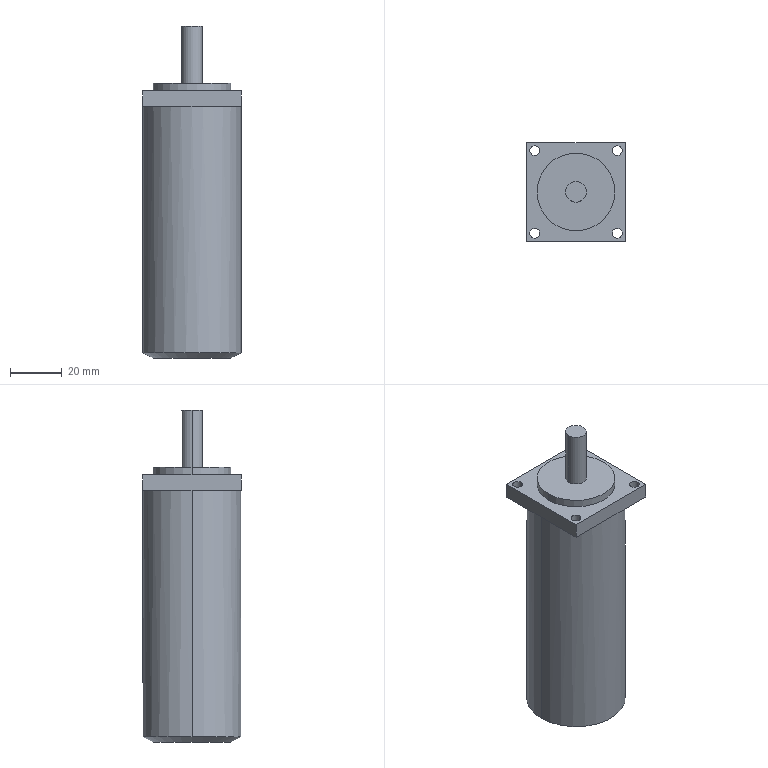Part | SolidWorks | features Boss 3, Chamfer 1, Cut 1, Extrusion 1 | 1 solid | 28 faces | box 38 x 38 x 128 mm | volume 121184 mm3 | cylinder 14 | plane 12 | cone 2 | commonest cylinder face diameters 3.797 x8 8 x2 30 x2 38 x2
STEP:
#1=CARTESIAN_POINT('',(4.,19.,-97.));
#2=VERTEX_POINT('',#1);
#3=CARTESIAN_POINT('',(34.,19.,-97.));
#4=VERTEX_POINT('',#3);
#5=CARTESIAN_POINT('',(19.,19.,-97.));
#6=DIRECTION('',(0.,0.,-1.));
#7=DIRECTION('',(-1.,0.,0.));
#8=AXIS2_PLACEMENT_3D('',#5,#6,#7);
#9=CIRCLE('',#8,15.);
#10=EDGE_CURVE('',#2,#4,#9,.T.);
#11=ORIENTED_EDGE('',*,*,#10,.F.);
#12=CARTESIAN_POINT('',(0.,19.,-95.));
#13=VERTEX_POINT('',#12);
#14=CARTESIAN_POINT('',(4.,19.,-97.));
#15=DIRECTION('',(-0.8944,0.,0.4472));
#16=VECTOR('',#15,1000.);
#17=LINE('',#14,#16);
#18=EDGE_CURVE('',#2,#13,#17,.T.);
#19=ORIENTED_EDGE('',*,*,#18,.T.);
#20=CARTESIAN_POINT('',(38.,19.,-95.));
#21=VERTEX_POINT('',#20);
#22=CARTESIAN_POINT('',(19.,19.,-95.));
#23=DIRECTION('',(0.,0.,1.));
#24=DIRECTION('',(-1.,0.,0.));
#25=AXIS2_PLACEMENT_3D('',#22,#23,#24);
#26=CIRCLE('',#25,19.);
#27=EDGE_CURVE('',#21,#13,#26,.T.);
#28=ORIENTED_EDGE('',*,*,#27,.F.);
#29=CARTESIAN_POINT('',(34.,19.,-97.));
#30=DIRECTION('',(0.8944,0.,0.4472));
#31=VECTOR('',#30,1000.);
#32=LINE('',#29,#31);
#33=EDGE_CURVE('',#4,#21,#32,.T.);
#34=ORIENTED_EDGE('',*,*,#33,.F.);
#35=EDGE_LOOP('',(#11,#19,#28,#34));
#36=FACE_OUTER_BOUND('',#35,.T.);
#37=CARTESIAN_POINT('',(19.,19.,-97.));
#38=DIRECTION('',(0.,0.,1.));
#39=DIRECTION('',(1.,0.,0.));
#40=AXIS2_PLACEMENT_3D('',#37,#38,#39);
#41=CONICAL_SURFACE('',#40,15.,1.107);
#42=ADVANCED_FACE('',(#36),#41,.T.);
#43=CARTESIAN_POINT('',(1.191,3.09,0.));
#44=VERTEX_POINT('',#43);
#45=CARTESIAN_POINT('',(4.989,3.09,0.));
#46=VERTEX_POINT('',#45);
#47=CARTESIAN_POINT('',(3.09,3.09,0.));
#48=DIRECTION('',(0.,0.,1.));
#49=DIRECTION('',(-1.,0.,0.));
#50=AXIS2_PLACEMENT_3D('',#47,#48,#49);
#51=CIRCLE('',#50,1.899);
#52=EDGE_CURVE('',#44,#46,#51,.T.);
#53=ORIENTED_EDGE('',*,*,#52,.F.);
#54=CARTESIAN_POINT('',(1.191,3.09,6.));
#55=VERTEX_POINT('',#54);
#56=CARTESIAN_POINT('',(1.191,3.09,-97.001));
#57=DIRECTION('',(0.,0.,1.));
#58=VECTOR('',#57,1000.);
#59=LINE('',#56,#58);
#60=EDGE_CURVE('',#44,#55,#59,.T.);
#61=ORIENTED_EDGE('',*,*,#60,.T.);
#62=CARTESIAN_POINT('',(4.989,3.09,6.));
#63=VERTEX_POINT('',#62);
#64=CARTESIAN_POINT('',(3.09,3.09,6.));
#65=DIRECTION('',(0.,0.,1.));
#66=DIRECTION('',(1.,0.,0.));
#67=AXIS2_PLACEMENT_3D('',#64,#65,#66);
#68=CIRCLE('',#67,1.899);
#69=EDGE_CURVE('',#55,#63,#68,.T.);
#70=ORIENTED_EDGE('',*,*,#69,.T.);
#71=CARTESIAN_POINT('',(4.989,3.09,-97.001));
#72=DIRECTION('',(0.,0.,1.));
#73=VECTOR('',#72,1000.);
#74=LINE('',#71,#73);
#75=EDGE_CURVE('',#46,#63,#74,.T.);
#76=ORIENTED_EDGE('',*,*,#75,.F.);
#77=EDGE_LOOP('',(#53,#61,#70,#76));
#78=FACE_OUTER_BOUND('',#77,.T.);
#79=CARTESIAN_POINT('',(3.09,3.09,-97.001));
#80=DIRECTION('',(0.,0.,1.));
#81=DIRECTION('',(1.,0.,0.));
#82=AXIS2_PLACEMENT_3D('',#79,#80,#81);
#83=CYLINDRICAL_SURFACE('',#82,1.899);
#84=ADVANCED_FACE('',(#78),#83,.F.);
#85=CARTESIAN_POINT('',(33.011,3.09,0.));
#86=VERTEX_POINT('',#85);
#87=CARTESIAN_POINT('',(36.809,3.09,0.));
#88=VERTEX_POINT('',#87);
#89=CARTESIAN_POINT('',(34.91,3.09,0.));
#90=DIRECTION('',(0.,0.,1.));
#91=DIRECTION('',(-1.,0.,0.));
#92=AXIS2_PLACEMENT_3D('',#89,#90,#91);
#93=CIRCLE('',#92,1.899);
#94=EDGE_CURVE('',#86,#88,#93,.T.);
#95=ORIENTED_EDGE('',*,*,#94,.F.);
#96=CARTESIAN_POINT('',(33.011,3.09,6.));
#97=VERTEX_POINT('',#96);
#98=CARTESIAN_POINT('',(33.011,3.09,-97.001));
#99=DIRECTION('',(0.,0.,1.));
#100=VECTOR('',#99,1000.);
#101=LINE('',#98,#100);
#102=EDGE_CURVE('',#86,#97,#101,.T.);
#103=ORIENTED_EDGE('',*,*,#102,.T.);
#104=CARTESIAN_POINT('',(36.809,3.09,6.));
#105=VERTEX_POINT('',#104);
#106=CARTESIAN_POINT('',(34.91,3.09,6.));
#107=DIRECTION('',(0.,0.,1.));
#108=DIRECTION('',(1.,0.,0.));
#109=AXIS2_PLACEMENT_3D('',#106,#107,#108);
#110=CIRCLE('',#109,1.899);
#111=EDGE_CURVE('',#97,#105,#110,.T.);
#112=ORIENTED_EDGE('',*,*,#111,.T.);
#113=CARTESIAN_POINT('',(36.809,3.09,-97.001));
#114=DIRECTION('',(0.,0.,1.));
#115=VECTOR('',#114,1000.);
#116=LINE('',#113,#115);
#117=EDGE_CURVE('',#88,#105,#116,.T.);
#118=ORIENTED_EDGE('',*,*,#117,.F.);
#119=EDGE_LOOP('',(#95,#103,#112,#118));
#120=FACE_OUTER_BOUND('',#119,.T.);
#121=CARTESIAN_POINT('',(34.91,3.09,-97.001));
#122=DIRECTION('',(0.,0.,1.));
#123=DIRECTION('',(1.,0.,0.));
#124=AXIS2_PLACEMENT_3D('',#121,#122,#123);
#125=CYLINDRICAL_SURFACE('',#124,1.899);
#126=ADVANCED_FACE('',(#120),#125,.F.);
#127=CARTESIAN_POINT('',(33.011,34.91,0.));
#128=VERTEX_POINT('',#127);
#129=CARTESIAN_POINT('',(36.809,34.91,0.));
#130=VERTEX_POINT('',#129);
#131=CARTESIAN_POINT('',(34.91,34.91,0.));
#132=DIRECTION('',(0.,0.,1.));
#133=DIRECTION('',(-1.,0.,0.));
#134=AXIS2_PLACEMENT_3D('',#131,#132,#133);
#135=CIRCLE('',#134,1.899);
#136=EDGE_CURVE('',#128,#130,#135,.T.);
#137=ORIENTED_EDGE('',*,*,#136,.F.);
#138=CARTESIAN_POINT('',(33.011,34.91,6.));
#139=VERTEX_POINT('',#138);
#140=CARTESIAN_POINT('',(33.011,34.91,-97.001));
#141=DIRECTION('',(0.,0.,1.));
#142=VECTOR('',#141,1000.);
#143=LINE('',#140,#142);
#144=EDGE_CURVE('',#128,#139,#143,.T.);
#145=ORIENTED_EDGE('',*,*,#144,.T.);
#146=CARTESIAN_POINT('',(36.809,34.91,6.));
#147=VERTEX_POINT('',#146);
#148=CARTESIAN_POINT('',(34.91,34.91,6.));
#149=DIRECTION('',(0.,0.,1.));
#150=DIRECTION('',(1.,0.,0.));
#151=AXIS2_PLACEMENT_3D('',#148,#149,#150);
#152=CIRCLE('',#151,1.899);
#153=EDGE_CURVE('',#139,#147,#152,.T.);
#154=ORIENTED_EDGE('',*,*,#153,.T.);
#155=CARTESIAN_POINT('',(36.809,34.91,-97.001));
#156=DIRECTION('',(0.,0.,1.));
#157=VECTOR('',#156,1000.);
#158=LINE('',#155,#157);
#159=EDGE_CURVE('',#130,#147,#158,.T.);
#160=ORIENTED_EDGE('',*,*,#159,.F.);
#161=EDGE_LOOP('',(#137,#145,#154,#160));
#162=FACE_OUTER_BOUND('',#161,.T.);
#163=CARTESIAN_POINT('',(34.91,34.91,-97.001));
#164=DIRECTION('',(0.,0.,1.));
#165=DIRECTION('',(1.,0.,0.));
#166=AXIS2_PLACEMENT_3D('',#163,#164,#165);
#167=CYLINDRICAL_SURFACE('',#166,1.899);
#168=ADVANCED_FACE('',(#162),#167,.F.);
#169=CARTESIAN_POINT('',(1.191,34.91,0.));
#170=VERTEX_POINT('',#169);
#171=CARTESIAN_POINT('',(4.989,34.91,0.));
#172=VERTEX_POINT('',#171);
#173=CARTESIAN_POINT('',(3.09,34.91,0.));
#174=DIRECTION('',(0.,0.,1.));
#175=DIRECTION('',(-1.,0.,0.));
#176=AXIS2_PLACEMENT_3D('',#173,#174,#175);
#177=CIRCLE('',#176,1.899);
#178=EDGE_CURVE('',#170,#172,#177,.T.);
#179=ORIENTED_EDGE('',*,*,#178,.F.);
#180=CARTESIAN_POINT('',(1.191,34.91,6.));
#181=VERTEX_POINT('',#180);
#182=CARTESIAN_POINT('',(1.191,34.91,-97.001));
#183=DIRECTION('',(0.,0.,1.));
#184=VECTOR('',#183,1000.);
#185=LINE('',#182,#184);
#186=EDGE_CURVE('',#170,#181,#185,.T.);
#187=ORIENTED_EDGE('',*,*,#186,.T.);
#188=CARTESIAN_POINT('',(4.989,34.91,6.));
#189=VERTEX_POINT('',#188);
#190=CARTESIAN_POINT('',(3.09,34.91,6.));
#191=DIRECTION('',(0.,0.,1.));
#192=DIRECTION('',(1.,0.,0.));
#193=AXIS2_PLACEMENT_3D('',#190,#191,#192);
#194=CIRCLE('',#193,1.899);
#195=EDGE_CURVE('',#181,#189,#194,.T.);
#196=ORIENTED_EDGE('',*,*,#195,.T.);
#197=CARTESIAN_POINT('',(4.989,34.91,-97.001));
#198=DIRECTION('',(0.,0.,1.));
#199=VECTOR('',#198,1000.);
#200=LINE('',#197,#199);
#201=EDGE_CURVE('',#172,#189,#200,.T.);
#202=ORIENTED_EDGE('',*,*,#201,.F.);
#203=EDGE_LOOP('',(#179,#187,#196,#202));
#204=FACE_OUTER_BOUND('',#203,.T.);
#205=CARTESIAN_POINT('',(3.09,34.91,-97.001));
#206=DIRECTION('',(0.,0.,1.));
#207=DIRECTION('',(1.,0.,0.));
#208=AXIS2_PLACEMENT_3D('',#205,#206,#207);
#209=CYLINDRICAL_SURFACE('',#208,1.899);
#210=ADVANCED_FACE('',(#204),#209,.F.);
#211=ORIENTED_EDGE('',*,*,#27,.T.);
#212=CARTESIAN_POINT('',(0.,19.,0.));
#213=VERTEX_POINT('',#212);
#214=CARTESIAN_POINT('',(0.,19.,-97.));
#215=DIRECTION('',(0.,0.,1.));
#216=VECTOR('',#215,1000.);
#217=LINE('',#214,#216);
#218=EDGE_CURVE('',#13,#213,#217,.T.);
#219=ORIENTED_EDGE('',*,*,#218,.T.);
#220=CARTESIAN_POINT('',(19.,38.,0.));
#221=VERTEX_POINT('',#220);
#222=CARTESIAN_POINT('',(19.,19.,0.));
#223=DIRECTION('',(0.,0.,-1.));
#224=DIRECTION('',(-1.,0.,0.));
#225=AXIS2_PLACEMENT_3D('',#222,#223,#224);
#226=CIRCLE('',#225,19.);
#227=EDGE_CURVE('',#213,#221,#226,.T.);
#228=ORIENTED_EDGE('',*,*,#227,.T.);
#229=CARTESIAN_POINT('',(38.,19.,0.));
#230=VERTEX_POINT('',#229);
#231=CARTESIAN_POINT('',(19.,19.,0.));
#232=DIRECTION('',(0.,0.,-1.));
#233=DIRECTION('',(-1.,0.,0.));
#234=AXIS2_PLACEMENT_3D('',#231,#232,#233);
#235=CIRCLE('',#234,19.);
#236=EDGE_CURVE('',#221,#230,#235,.T.);
#237=ORIENTED_EDGE('',*,*,#236,.T.);
#238=CARTESIAN_POINT('',(38.,19.,-97.));
#239=DIRECTION('',(0.,0.,1.));
#240=VECTOR('',#239,1000.);
#241=LINE('',#238,#240);
#242=EDGE_CURVE('',#21,#230,#241,.T.);
#243=ORIENTED_EDGE('',*,*,#242,.F.);
#244=EDGE_LOOP('',(#211,#219,#228,#237,#243));
#245=FACE_OUTER_BOUND('',#244,.T.);
#246=CARTESIAN_POINT('',(19.,19.,-97.));
#247=DIRECTION('',(0.,0.,1.));
#248=DIRECTION('',(1.,0.,0.));
#249=AXIS2_PLACEMENT_3D('',#246,#247,#248);
#250=CYLINDRICAL_SURFACE('',#249,19.);
#251=ADVANCED_FACE('',(#245),#250,.T.);
#252=CARTESIAN_POINT('',(23.,19.,31.));
#253=VERTEX_POINT('',#252);
#254=CARTESIAN_POINT('',(15.,19.,31.));
#255=VERTEX_POINT('',#254);
#256=CARTESIAN_POINT('',(19.,19.,31.));
#257=DIRECTION('',(0.,0.,1.));
#258=DIRECTION('',(1.,0.,0.));
#259=AXIS2_PLACEMENT_3D('',#256,#257,#258);
#260=CIRCLE('',#259,4.);
#261=EDGE_CURVE('',#253,#255,#260,.T.);
#262=ORIENTED_EDGE('',*,*,#261,.F.);
#263=CARTESIAN_POINT('',(23.,19.,9.));
#264=VERTEX_POINT('',#263);
#265=CARTESIAN_POINT('',(23.,19.,31.));
#266=DIRECTION('',(0.,0.,-1.));
#267=VECTOR('',#266,1000.);
#268=LINE('',#265,#267);
#269=EDGE_CURVE('',#253,#264,#268,.T.);
#270=ORIENTED_EDGE('',*,*,#269,.T.);
#271=CARTESIAN_POINT('',(15.,19.,9.));
#272=VERTEX_POINT('',#271);
#273=CARTESIAN_POINT('',(19.,19.,9.));
#274=DIRECTION('',(0.,0.,1.));
#275=DIRECTION('',(1.,0.,0.));
#276=AXIS2_PLACEMENT_3D('',#273,#274,#275);
#277=CIRCLE('',#276,4.);
#278=EDGE_CURVE('',#264,#272,#277,.T.);
#279=ORIENTED_EDGE('',*,*,#278,.T.);
#280=CARTESIAN_POINT('',(15.,19.,31.));
#281=DIRECTION('',(0.,0.,-1.));
#282=VECTOR('',#281,1000.);
#283=LINE('',#280,#282);
#284=EDGE_CURVE('',#255,#272,#283,.T.);
#285=ORIENTED_EDGE('',*,*,#284,.F.);
#286=EDGE_LOOP('',(#262,#270,#279,#285));
#287=FACE_OUTER_BOUND('',#286,.T.);
#288=CARTESIAN_POINT('',(19.,19.,31.));
#289=DIRECTION('',(0.,0.,-1.));
#290=DIRECTION('',(-1.,0.,0.));
#291=AXIS2_PLACEMENT_3D('',#288,#289,#290);
#292=CYLINDRICAL_SURFACE('',#291,4.);
#293=ADVANCED_FACE('',(#287),#292,.T.);
#294=CARTESIAN_POINT('',(34.,19.,9.));
#295=VERTEX_POINT('',#294);
#296=CARTESIAN_POINT('',(4.,19.,9.));
#297=VERTEX_POINT('',#296);
#298=CARTESIAN_POINT('',(19.,19.,9.));
#299=DIRECTION('',(0.,0.,1.));
#300=DIRECTION('',(1.,0.,0.));
#301=AXIS2_PLACEMENT_3D('',#298,#299,#300);
#302=CIRCLE('',#301,15.);
#303=EDGE_CURVE('',#295,#297,#302,.T.);
#304=ORIENTED_EDGE('',*,*,#303,.F.);
#305=CARTESIAN_POINT('',(34.,19.,6.));
#306=VERTEX_POINT('',#305);
#307=CARTESIAN_POINT('',(34.,19.,9.));
#308=DIRECTION('',(0.,0.,-1.));
#309=VECTOR('',#308,1000.);
#310=LINE('',#307,#309);
#311=EDGE_CURVE('',#295,#306,#310,.T.);
#312=ORIENTED_EDGE('',*,*,#311,.T.);
#313=CARTESIAN_POINT('',(4.,19.,6.));
#314=VERTEX_POINT('',#313);
#315=CARTESIAN_POINT('',(19.,19.,6.));
#316=DIRECTION('',(0.,0.,1.));
#317=DIRECTION('',(-1.,0.,0.));
#318=AXIS2_PLACEMENT_3D('',#315,#316,#317);
#319=CIRCLE('',#318,15.);
#320=EDGE_CURVE('',#306,#314,#319,.T.);
#321=ORIENTED_EDGE('',*,*,#320,.T.);
#322=CARTESIAN_POINT('',(4.,19.,9.));
#323=DIRECTION('',(0.,0.,-1.));
#324=VECTOR('',#323,1000.);
#325=LINE('',#322,#324);
#326=EDGE_CURVE('',#297,#314,#325,.T.);
#327=ORIENTED_EDGE('',*,*,#326,.F.);
#328=EDGE_LOOP('',(#304,#312,#321,#327));
#329=FACE_OUTER_BOUND('',#328,.T.);
#330=CARTESIAN_POINT('',(19.,19.,9.));
#331=DIRECTION('',(0.,0.,-1.));
#332=DIRECTION('',(-1.,0.,0.));
#333=AXIS2_PLACEMENT_3D('',#330,#331,#332);
#334=CYLINDRICAL_SURFACE('',#333,15.);
#335=ADVANCED_FACE('',(#329),#334,.T.);
#336=CARTESIAN_POINT('',(3.09,34.91,0.));
#337=DIRECTION('',(0.,0.,1.));
#338=DIRECTION('',(-1.,0.,0.));
#339=AXIS2_PLACEMENT_3D('',#336,#337,#338);
#340=CIRCLE('',#339,1.899);
#341=EDGE_CURVE('',#172,#170,#340,.T.);
#342=ORIENTED_EDGE('',*,*,#341,.T.);
#343=ORIENTED_EDGE('',*,*,#178,.T.);
#344=EDGE_LOOP('',(#342,#343));
#345=FACE_BOUND('',#344,.T.);
#346=ORIENTED_EDGE('',*,*,#227,.F.);
#347=CARTESIAN_POINT('',(0.,38.,0.));
#348=VERTEX_POINT('',#347);
#349=CARTESIAN_POINT('',(0.,0.,0.));
#350=DIRECTION('',(0.,-1.,0.));
#351=VECTOR('',#350,1000.);
#352=LINE('',#349,#351);
#353=EDGE_CURVE('',#348,#213,#352,.T.);
#354=ORIENTED_EDGE('',*,*,#353,.F.);
#355=CARTESIAN_POINT('',(0.,38.,0.));
#356=DIRECTION('',(-1.,0.,0.));
#357=VECTOR('',#356,1000.);
#358=LINE('',#355,#357);
#359=EDGE_CURVE('',#221,#348,#358,.T.);
#360=ORIENTED_EDGE('',*,*,#359,.F.);
#361=EDGE_LOOP('',(#346,#354,#360));
#362=FACE_OUTER_BOUND('',#361,.T.);
#363=CARTESIAN_POINT('',(0.,38.,0.));
#364=DIRECTION('',(0.,0.,-1.));
#365=DIRECTION('',(-1.,0.,0.));
#366=AXIS2_PLACEMENT_3D('',#363,#364,#365);
#367=PLANE('',#366);
#368=ADVANCED_FACE('',(#345,#362),#367,.T.);
#369=CARTESIAN_POINT('',(34.91,34.91,0.));
#370=DIRECTION('',(0.,0.,1.));
#371=DIRECTION('',(-1.,0.,0.));
#372=AXIS2_PLACEMENT_3D('',#369,#370,#371);
#373=CIRCLE('',#372,1.899);
#374=EDGE_CURVE('',#130,#128,#373,.T.);
#375=ORIENTED_EDGE('',*,*,#374,.T.);
#376=ORIENTED_EDGE('',*,*,#136,.T.);
#377=EDGE_LOOP('',(#375,#376));
#378=FACE_BOUND('',#377,.T.);
#379=ORIENTED_EDGE('',*,*,#236,.F.);
#380=CARTESIAN_POINT('',(38.,38.,0.));
#381=VERTEX_POINT('',#380);
#382=CARTESIAN_POINT('',(0.,38.,0.));
#383=DIRECTION('',(-1.,0.,0.));
#384=VECTOR('',#383,1000.);
#385=LINE('',#382,#384);
#386=EDGE_CURVE('',#381,#221,#385,.T.);
#387=ORIENTED_EDGE('',*,*,#386,.F.);
#388=CARTESIAN_POINT('',(38.,0.,0.));
#389=DIRECTION('',(0.,1.,0.));
#390=VECTOR('',#389,1000.);
#391=LINE('',#388,#390);
#392=EDGE_CURVE('',#230,#381,#391,.T.);
#393=ORIENTED_EDGE('',*,*,#392,.F.);
#394=EDGE_LOOP('',(#379,#387,#393));
#395=FACE_OUTER_BOUND('',#394,.T.);
#396=CARTESIAN_POINT('',(0.,38.,0.));
#397=DIRECTION('',(0.,0.,-1.));
#398=DIRECTION('',(-1.,0.,0.));
#399=AXIS2_PLACEMENT_3D('',#396,#397,#398);
#400=PLANE('',#399);
#401=ADVANCED_FACE('',(#378,#395),#400,.T.);
#402=CARTESIAN_POINT('',(34.91,3.09,0.));
#403=DIRECTION('',(0.,0.,1.));
#404=DIRECTION('',(-1.,0.,0.));
#405=AXIS2_PLACEMENT_3D('',#402,#403,#404);
#406=CIRCLE('',#405,1.899);
#407=EDGE_CURVE('',#88,#86,#406,.T.);
#408=ORIENTED_EDGE('',*,*,#407,.T.);
#409=ORIENTED_EDGE('',*,*,#94,.T.);
#410=EDGE_LOOP('',(#408,#409));
#411=FACE_BOUND('',#410,.T.);
#412=CARTESIAN_POINT('',(19.,0.,0.));
#413=VERTEX_POINT('',#412);
#414=CARTESIAN_POINT('',(19.,19.,0.));
#415=DIRECTION('',(0.,0.,-1.));
#416=DIRECTION('',(-1.,0.,0.));
#417=AXIS2_PLACEMENT_3D('',#414,#415,#416);
#418=CIRCLE('',#417,19.);
#419=EDGE_CURVE('',#230,#413,#418,.T.);
#420=ORIENTED_EDGE('',*,*,#419,.F.);
#421=CARTESIAN_POINT('',(38.,0.,0.));
#422=VERTEX_POINT('',#421);
#423=CARTESIAN_POINT('',(38.,0.,0.));
#424=DIRECTION('',(0.,1.,0.));
#425=VECTOR('',#424,1000.);
#426=LINE('',#423,#425);
#427=EDGE_CURVE('',#422,#230,#426,.T.);
#428=ORIENTED_EDGE('',*,*,#427,.F.);
#429=CARTESIAN_POINT('',(0.,0.,0.));
#430=DIRECTION('',(1.,0.,0.));
#431=VECTOR('',#430,1000.);
#432=LINE('',#429,#431);
#433=EDGE_CURVE('',#413,#422,#432,.T.);
#434=ORIENTED_EDGE('',*,*,#433,.F.);
#435=EDGE_LOOP('',(#420,#428,#434));
#436=FACE_OUTER_BOUND('',#435,.T.);
#437=CARTESIAN_POINT('',(0.,38.,0.));
#438=DIRECTION('',(0.,0.,-1.));
#439=DIRECTION('',(-1.,0.,0.));
#440=AXIS2_PLACEMENT_3D('',#437,#438,#439);
#441=PLANE('',#440);
#442=ADVANCED_FACE('',(#411,#436),#441,.T.);
#443=CARTESIAN_POINT('',(19.,19.,9.));
#444=DIRECTION('',(0.,0.,1.));
#445=DIRECTION('',(1.,0.,0.));
#446=AXIS2_PLACEMENT_3D('',#443,#444,#445);
#447=CIRCLE('',#446,15.);
#448=EDGE_CURVE('',#297,#295,#447,.T.);
#449=ORIENTED_EDGE('',*,*,#448,.T.);
#450=ORIENTED_EDGE('',*,*,#303,.T.);
#451=EDGE_LOOP('',(#449,#450));
#452=FACE_OUTER_BOUND('',#451,.T.);
#453=CARTESIAN_POINT('',(19.,19.,9.));
#454=DIRECTION('',(0.,0.,1.));
#455=DIRECTION('',(1.,0.,0.));
#456=AXIS2_PLACEMENT_3D('',#453,#454,#455);
#457=CIRCLE('',#456,4.);
#458=EDGE_CURVE('',#272,#264,#457,.T.);
#459=ORIENTED_EDGE('',*,*,#458,.F.);
#460=ORIENTED_EDGE('',*,*,#278,.F.);
#461=EDGE_LOOP('',(#459,#460));
#462=FACE_BOUND('',#461,.T.);
#463=CARTESIAN_POINT('',(19.,19.,9.));
#464=DIRECTION('',(0.,0.,1.));
#465=DIRECTION('',(1.,0.,0.));
#466=AXIS2_PLACEMENT_3D('',#463,#464,#465);
#467=PLANE('',#466);
#468=ADVANCED_FACE('',(#452,#462),#467,.T.);
#469=CARTESIAN_POINT('',(3.09,3.09,6.));
#470=DIRECTION('',(0.,0.,1.));
#471=DIRECTION('',(1.,0.,0.));
#472=AXIS2_PLACEMENT_3D('',#469,#470,#471);
#473=CIRCLE('',#472,1.899);
#474=EDGE_CURVE('',#63,#55,#473,.T.);
#475=ORIENTED_EDGE('',*,*,#474,.F.);
#476=ORIENTED_EDGE('',*,*,#69,.F.);
#477=EDGE_LOOP('',(#475,#476));
#478=FACE_BOUND('',#477,.T.);
#479=CARTESIAN_POINT('',(34.91,3.09,6.));
#480=DIRECTION('',(0.,0.,1.));
#481=DIRECTION('',(1.,0.,0.));
#482=AXIS2_PLACEMENT_3D('',#479,#480,#481);
#483=CIRCLE('',#482,1.899);
#484=EDGE_CURVE('',#105,#97,#483,.T.);
#485=ORIENTED_EDGE('',*,*,#484,.F.);
#486=ORIENTED_EDGE('',*,*,#111,.F.);
#487=EDGE_LOOP('',(#485,#486));
#488=FACE_BOUND('',#487,.T.);
#489=CARTESIAN_POINT('',(34.91,34.91,6.));
#490=DIRECTION('',(0.,0.,1.));
#491=DIRECTION('',(1.,0.,0.));
#492=AXIS2_PLACEMENT_3D('',#489,#490,#491);
#493=CIRCLE('',#492,1.899);
#494=EDGE_CURVE('',#147,#139,#493,.T.);
#495=ORIENTED_EDGE('',*,*,#494,.F.);
#496=ORIENTED_EDGE('',*,*,#153,.F.);
#497=EDGE_LOOP('',(#495,#496));
#498=FACE_BOUND('',#497,.T.);
#499=CARTESIAN_POINT('',(3.09,34.91,6.));
#500=DIRECTION('',(0.,0.,1.));
#501=DIRECTION('',(1.,0.,0.));
#502=AXIS2_PLACEMENT_3D('',#499,#500,#501);
#503=CIRCLE('',#502,1.899);
#504=EDGE_CURVE('',#189,#181,#503,.T.);
#505=ORIENTED_EDGE('',*,*,#504,.F.);
#506=ORIENTED_EDGE('',*,*,#195,.F.);
#507=EDGE_LOOP('',(#505,#506));
#508=FACE_BOUND('',#507,.T.);
#509=CARTESIAN_POINT('',(0.,38.,6.));
#510=VERTEX_POINT('',#509);
#511=CARTESIAN_POINT('',(0.,0.,6.));
#512=VERTEX_POINT('',#511);
#513=CARTESIAN_POINT('',(0.,0.,6.));
#514=DIRECTION('',(0.,-1.,0.));
#515=VECTOR('',#514,1000.);
#516=LINE('',#513,#515);
#517=EDGE_CURVE('',#510,#512,#516,.T.);
#518=ORIENTED_EDGE('',*,*,#517,.T.);
#519=CARTESIAN_POINT('',(38.,0.,6.));
#520=VERTEX_POINT('',#519);
#521=CARTESIAN_POINT('',(0.,0.,6.));
#522=DIRECTION('',(1.,0.,0.));
#523=VECTOR('',#522,1000.);
#524=LINE('',#521,#523);
#525=EDGE_CURVE('',#512,#520,#524,.T.);
#526=ORIENTED_EDGE('',*,*,#525,.T.);
#527=CARTESIAN_POINT('',(38.,38.,6.));
#528=VERTEX_POINT('',#527);
#529=CARTESIAN_POINT('',(38.,0.,6.));
#530=DIRECTION('',(0.,1.,0.));
#531=VECTOR('',#530,1000.);
#532=LINE('',#529,#531);
#533=EDGE_CURVE('',#520,#528,#532,.T.);
#534=ORIENTED_EDGE('',*,*,#533,.T.);
#535=CARTESIAN_POINT('',(0.,38.,6.));
#536=DIRECTION('',(-1.,0.,0.));
#537=VECTOR('',#536,1000.);
#538=LINE('',#535,#537);
#539=EDGE_CURVE('',#528,#510,#538,.T.);
#540=ORIENTED_EDGE('',*,*,#539,.T.);
#541=EDGE_LOOP('',(#518,#526,#534,#540));
#542=FACE_OUTER_BOUND('',#541,.T.);
#543=CARTESIAN_POINT('',(19.,19.,6.));
#544=DIRECTION('',(0.,0.,1.));
#545=DIRECTION('',(-1.,0.,0.));
#546=AXIS2_PLACEMENT_3D('',#543,#544,#545);
#547=CIRCLE('',#546,15.);
#548=EDGE_CURVE('',#314,#306,#547,.T.);
#549=ORIENTED_EDGE('',*,*,#548,.F.);
#550=ORIENTED_EDGE('',*,*,#320,.F.);
#551=EDGE_LOOP('',(#549,#550));
#552=FACE_BOUND('',#551,.T.);
#553=CARTESIAN_POINT('',(0.,38.,6.));
#554=DIRECTION('',(0.,0.,-1.));
#555=DIRECTION('',(-1.,0.,0.));
#556=AXIS2_PLACEMENT_3D('',#553,#554,#555);
#557=PLANE('',#556);
#558=ADVANCED_FACE('',(#478,#488,#498,#508,#542,#552),#557,.F.);
#559=ORIENTED_EDGE('',*,*,#353,.T.);
#560=CARTESIAN_POINT('',(0.,0.,0.));
#561=VERTEX_POINT('',#560);
#562=CARTESIAN_POINT('',(0.,0.,0.));
#563=DIRECTION('',(0.,-1.,0.));
#564=VECTOR('',#563,1000.);
#565=LINE('',#562,#564);
#566=EDGE_CURVE('',#213,#561,#565,.T.);
#567=ORIENTED_EDGE('',*,*,#566,.T.);
#568=CARTESIAN_POINT('',(0.,0.,6.));
#569=DIRECTION('',(0.,0.,-1.));
#570=VECTOR('',#569,1000.);
#571=LINE('',#568,#570);
#572=EDGE_CURVE('',#512,#561,#571,.T.);
#573=ORIENTED_EDGE('',*,*,#572,.F.);
#574=ORIENTED_EDGE('',*,*,#517,.F.);
#575=CARTESIAN_POINT('',(0.,38.,6.));
#576=DIRECTION('',(0.,0.,-1.));
#577=VECTOR('',#576,1000.);
#578=LINE('',#575,#577);
#579=EDGE_CURVE('',#510,#348,#578,.T.);
#580=ORIENTED_EDGE('',*,*,#579,.T.);
#581=EDGE_LOOP('',(#559,#567,#573,#574,#580));
#582=FACE_OUTER_BOUND('',#581,.T.);
#583=CARTESIAN_POINT('',(0.,0.,6.));
#584=DIRECTION('',(1.,0.,0.));
#585=DIRECTION('',(0.,0.,-1.));
#586=AXIS2_PLACEMENT_3D('',#583,#584,#585);
#587=PLANE('',#586);
#588=ADVANCED_FACE('',(#582),#587,.F.);
#589=CARTESIAN_POINT('',(0.,0.,0.));
#590=DIRECTION('',(1.,0.,0.));
#591=VECTOR('',#590,1000.);
#592=LINE('',#589,#591);
#593=EDGE_CURVE('',#561,#413,#592,.T.);
#594=ORIENTED_EDGE('',*,*,#593,.T.);
#595=ORIENTED_EDGE('',*,*,#433,.T.);
#596=CARTESIAN_POINT('',(38.,0.,6.));
#597=DIRECTION('',(0.,0.,-1.));
#598=VECTOR('',#597,1000.);
#599=LINE('',#596,#598);
#600=EDGE_CURVE('',#520,#422,#599,.T.);
#601=ORIENTED_EDGE('',*,*,#600,.F.);
#602=ORIENTED_EDGE('',*,*,#525,.F.);
#603=ORIENTED_EDGE('',*,*,#572,.T.);
#604=EDGE_LOOP('',(#594,#595,#601,#602,#603));
#605=FACE_OUTER_BOUND('',#604,.T.);
#606=CARTESIAN_POINT('',(0.,0.,6.));
#607=DIRECTION('',(0.,1.,0.));
#608=DIRECTION('',(0.,0.,1.));
#609=AXIS2_PLACEMENT_3D('',#606,#607,#608);
#610=PLANE('',#609);
#611=ADVANCED_FACE('',(#605),#610,.F.);
#612=ORIENTED_EDGE('',*,*,#427,.T.);
#613=ORIENTED_EDGE('',*,*,#392,.T.);
#614=CARTESIAN_POINT('',(38.,38.,6.));
#615=DIRECTION('',(0.,0.,-1.));
#616=VECTOR('',#615,1000.);
#617=LINE('',#614,#616);
#618=EDGE_CURVE('',#528,#381,#617,.T.);
#619=ORIENTED_EDGE('',*,*,#618,.F.);
#620=ORIENTED_EDGE('',*,*,#533,.F.);
#621=ORIENTED_EDGE('',*,*,#600,.T.);
#622=EDGE_LOOP('',(#612,#613,#619,#620,#621));
#623=FACE_OUTER_BOUND('',#622,.T.);
#624=CARTESIAN_POINT('',(38.,0.,6.));
#625=DIRECTION('',(-1.,0.,0.));
#626=DIRECTION('',(0.,0.,1.));
#627=AXIS2_PLACEMENT_3D('',#624,#625,#626);
#628=PLANE('',#627);
#629=ADVANCED_FACE('',(#623),#628,.F.);
#630=ORIENTED_EDGE('',*,*,#386,.T.);
#631=ORIENTED_EDGE('',*,*,#359,.T.);
#632=ORIENTED_EDGE('',*,*,#579,.F.);
#633=ORIENTED_EDGE('',*,*,#539,.F.);
#634=ORIENTED_EDGE('',*,*,#618,.T.);
#635=EDGE_LOOP('',(#630,#631,#632,#633,#634));
#636=FACE_OUTER_BOUND('',#635,.T.);
#637=CARTESIAN_POINT('',(0.,38.,6.));
#638=DIRECTION('',(0.,-1.,0.));
#639=DIRECTION('',(0.,0.,-1.));
#640=AXIS2_PLACEMENT_3D('',#637,#638,#639);
#641=PLANE('',#640);
#642=ADVANCED_FACE('',(#636),#641,.F.);
#643=CARTESIAN_POINT('',(3.09,3.09,0.));
#644=DIRECTION('',(0.,0.,1.));
#645=DIRECTION('',(-1.,0.,0.));
#646=AXIS2_PLACEMENT_3D('',#643,#644,#645);
#647=CIRCLE('',#646,1.899);
#648=EDGE_CURVE('',#46,#44,#647,.T.);
#649=ORIENTED_EDGE('',*,*,#648,.T.);
#650=ORIENTED_EDGE('',*,*,#52,.T.);
#651=EDGE_LOOP('',(#649,#650));
#652=FACE_BOUND('',#651,.T.);
#653=CARTESIAN_POINT('',(19.,19.,0.));
#654=DIRECTION('',(0.,0.,-1.));
#655=DIRECTION('',(-1.,0.,0.));
#656=AXIS2_PLACEMENT_3D('',#653,#654,#655);
#657=CIRCLE('',#656,19.);
#658=EDGE_CURVE('',#413,#213,#657,.T.);
#659=ORIENTED_EDGE('',*,*,#658,.F.);
#660=ORIENTED_EDGE('',*,*,#593,.F.);
#661=ORIENTED_EDGE('',*,*,#566,.F.);
#662=EDGE_LOOP('',(#659,#660,#661));
#663=FACE_OUTER_BOUND('',#662,.T.);
#664=CARTESIAN_POINT('',(0.,38.,0.));
#665=DIRECTION('',(0.,0.,-1.));
#666=DIRECTION('',(-1.,0.,0.));
#667=AXIS2_PLACEMENT_3D('',#664,#665,#666);
#668=PLANE('',#667);
#669=ADVANCED_FACE('',(#652,#663),#668,.T.);
#670=ORIENTED_EDGE('',*,*,#311,.F.);
#671=ORIENTED_EDGE('',*,*,#448,.F.);
#672=ORIENTED_EDGE('',*,*,#326,.T.);
#673=ORIENTED_EDGE('',*,*,#548,.T.);
#674=EDGE_LOOP('',(#670,#671,#672,#673));
#675=FACE_OUTER_BOUND('',#674,.T.);
#676=CARTESIAN_POINT('',(19.,19.,9.));
#677=DIRECTION('',(0.,0.,-1.));
#678=DIRECTION('',(-1.,0.,0.));
#679=AXIS2_PLACEMENT_3D('',#676,#677,#678);
#680=CYLINDRICAL_SURFACE('',#679,15.);
#681=ADVANCED_FACE('',(#675),#680,.T.);
#682=ORIENTED_EDGE('',*,*,#269,.F.);
#683=CARTESIAN_POINT('',(19.,19.,31.));
#684=DIRECTION('',(0.,0.,1.));
#685=DIRECTION('',(1.,0.,0.));
#686=AXIS2_PLACEMENT_3D('',#683,#684,#685);
#687=CIRCLE('',#686,4.);
#688=EDGE_CURVE('',#255,#253,#687,.T.);
#689=ORIENTED_EDGE('',*,*,#688,.F.);
#690=ORIENTED_EDGE('',*,*,#284,.T.);
#691=ORIENTED_EDGE('',*,*,#458,.T.);
#692=EDGE_LOOP('',(#682,#689,#690,#691));
#693=FACE_OUTER_BOUND('',#692,.T.);
#694=CARTESIAN_POINT('',(19.,19.,31.));
#695=DIRECTION('',(0.,0.,-1.));
#696=DIRECTION('',(-1.,0.,0.));
#697=AXIS2_PLACEMENT_3D('',#694,#695,#696);
#698=CYLINDRICAL_SURFACE('',#697,4.);
#699=ADVANCED_FACE('',(#693),#698,.T.);
#700=ORIENTED_EDGE('',*,*,#688,.T.);
#701=ORIENTED_EDGE('',*,*,#261,.T.);
#702=EDGE_LOOP('',(#700,#701));
#703=FACE_OUTER_BOUND('',#702,.T.);
#704=CARTESIAN_POINT('',(19.,19.,31.));
#705=DIRECTION('',(0.,0.,1.));
#706=DIRECTION('',(1.,0.,0.));
#707=AXIS2_PLACEMENT_3D('',#704,#705,#706);
#708=PLANE('',#707);
#709=ADVANCED_FACE('',(#703),#708,.T.);
#710=ORIENTED_EDGE('',*,*,#218,.F.);
#711=CARTESIAN_POINT('',(19.,19.,-95.));
#712=DIRECTION('',(0.,0.,1.));
#713=DIRECTION('',(-1.,0.,0.));
#714=AXIS2_PLACEMENT_3D('',#711,#712,#713);
#715=CIRCLE('',#714,19.);
#716=EDGE_CURVE('',#13,#21,#715,.T.);
#717=ORIENTED_EDGE('',*,*,#716,.T.);
#718=ORIENTED_EDGE('',*,*,#242,.T.);
#719=ORIENTED_EDGE('',*,*,#419,.T.);
#720=ORIENTED_EDGE('',*,*,#658,.T.);
#721=EDGE_LOOP('',(#710,#717,#718,#719,#720));
#722=FACE_OUTER_BOUND('',#721,.T.);
#723=CARTESIAN_POINT('',(19.,19.,-97.));
#724=DIRECTION('',(0.,0.,1.));
#725=DIRECTION('',(1.,0.,0.));
#726=AXIS2_PLACEMENT_3D('',#723,#724,#725);
#727=CYLINDRICAL_SURFACE('',#726,19.);
#728=ADVANCED_FACE('',(#722),#727,.T.);
#729=CARTESIAN_POINT('',(19.,19.,-97.));
#730=DIRECTION('',(0.,0.,-1.));
#731=DIRECTION('',(-1.,0.,0.));
#732=AXIS2_PLACEMENT_3D('',#729,#730,#731);
#733=CIRCLE('',#732,15.);
#734=EDGE_CURVE('',#4,#2,#733,.T.);
#735=ORIENTED_EDGE('',*,*,#734,.T.);
#736=ORIENTED_EDGE('',*,*,#10,.T.);
#737=EDGE_LOOP('',(#735,#736));
#738=FACE_OUTER_BOUND('',#737,.T.);
#739=CARTESIAN_POINT('',(19.,19.,-97.));
#740=DIRECTION('',(0.,0.,-1.));
#741=DIRECTION('',(-1.,0.,0.));
#742=AXIS2_PLACEMENT_3D('',#739,#740,#741);
#743=PLANE('',#742);
#744=ADVANCED_FACE('',(#738),#743,.T.);
#745=ORIENTED_EDGE('',*,*,#186,.F.);
#746=ORIENTED_EDGE('',*,*,#341,.F.);
#747=ORIENTED_EDGE('',*,*,#201,.T.);
#748=ORIENTED_EDGE('',*,*,#504,.T.);
#749=EDGE_LOOP('',(#745,#746,#747,#748));
#750=FACE_OUTER_BOUND('',#749,.T.);
#751=CARTESIAN_POINT('',(3.09,34.91,-97.001));
#752=DIRECTION('',(0.,0.,1.));
#753=DIRECTION('',(1.,0.,0.));
#754=AXIS2_PLACEMENT_3D('',#751,#752,#753);
#755=CYLINDRICAL_SURFACE('',#754,1.899);
#756=ADVANCED_FACE('',(#750),#755,.F.);
#757=ORIENTED_EDGE('',*,*,#144,.F.);
#758=ORIENTED_EDGE('',*,*,#374,.F.);
#759=ORIENTED_EDGE('',*,*,#159,.T.);
#760=ORIENTED_EDGE('',*,*,#494,.T.);
#761=EDGE_LOOP('',(#757,#758,#759,#760));
#762=FACE_OUTER_BOUND('',#761,.T.);
#763=CARTESIAN_POINT('',(34.91,34.91,-97.001));
#764=DIRECTION('',(0.,0.,1.));
#765=DIRECTION('',(1.,0.,0.));
#766=AXIS2_PLACEMENT_3D('',#763,#764,#765);
#767=CYLINDRICAL_SURFACE('',#766,1.899);
#768=ADVANCED_FACE('',(#762),#767,.F.);
#769=ORIENTED_EDGE('',*,*,#102,.F.);
#770=ORIENTED_EDGE('',*,*,#407,.F.);
#771=ORIENTED_EDGE('',*,*,#117,.T.);
#772=ORIENTED_EDGE('',*,*,#484,.T.);
#773=EDGE_LOOP('',(#769,#770,#771,#772));
#774=FACE_OUTER_BOUND('',#773,.T.);
#775=CARTESIAN_POINT('',(34.91,3.09,-97.001));
#776=DIRECTION('',(0.,0.,1.));
#777=DIRECTION('',(1.,0.,0.));
#778=AXIS2_PLACEMENT_3D('',#775,#776,#777);
#779=CYLINDRICAL_SURFACE('',#778,1.899);
#780=ADVANCED_FACE('',(#774),#779,.F.);
#781=ORIENTED_EDGE('',*,*,#60,.F.);
#782=ORIENTED_EDGE('',*,*,#648,.F.);
#783=ORIENTED_EDGE('',*,*,#75,.T.);
#784=ORIENTED_EDGE('',*,*,#474,.T.);
#785=EDGE_LOOP('',(#781,#782,#783,#784));
#786=FACE_OUTER_BOUND('',#785,.T.);
#787=CARTESIAN_POINT('',(3.09,3.09,-97.001));
#788=DIRECTION('',(0.,0.,1.));
#789=DIRECTION('',(1.,0.,0.));
#790=AXIS2_PLACEMENT_3D('',#787,#788,#789);
#791=CYLINDRICAL_SURFACE('',#790,1.899);
#792=ADVANCED_FACE('',(#786),#791,.F.);
#793=ORIENTED_EDGE('',*,*,#18,.F.);
#794=ORIENTED_EDGE('',*,*,#734,.F.);
#795=ORIENTED_EDGE('',*,*,#33,.T.);
#796=ORIENTED_EDGE('',*,*,#716,.F.);
#797=EDGE_LOOP('',(#793,#794,#795,#796));
#798=FACE_OUTER_BOUND('',#797,.T.);
#799=CARTESIAN_POINT('',(19.,19.,-97.));
#800=DIRECTION('',(0.,0.,1.));
#801=DIRECTION('',(1.,0.,0.));
#802=AXIS2_PLACEMENT_3D('',#799,#800,#801);
#803=CONICAL_SURFACE('',#802,15.,1.107);
#804=ADVANCED_FACE('',(#798),#803,.T.);
#805=CLOSED_SHELL('',(#42,#84,#126,#168,#210,#251,#293,#335,#368,#401,#442,#468,#558,#588,#611,#629,#642,#669,#681,#699,#709,#728,#744,#756,#768,#780,#792,#804));
#806=MANIFOLD_SOLID_BREP('',#805);
#807=CARTESIAN_POINT('',(0.,0.,0.));
#808=DIRECTION('',(0.,0.,1.));
#809=DIRECTION('',(1.,0.,0.));
#810=AXIS2_PLACEMENT_3D('',#807,#808,#809);
#811=(LENGTH_UNIT()NAMED_UNIT(*)SI_UNIT(.MILLI.,.METRE.));
#812=UNCERTAINTY_MEASURE_WITH_UNIT(LENGTH_MEASURE(0.00001),#811,'','');
#813=(NAMED_UNIT(*)PLANE_ANGLE_UNIT()SI_UNIT($,.RADIAN.));
#814=(NAMED_UNIT(*)SI_UNIT($,.STERADIAN.)SOLID_ANGLE_UNIT());
#815=(GEOMETRIC_REPRESENTATION_CONTEXT(3)GLOBAL_UNCERTAINTY_ASSIGNED_CONTEXT((#812))GLOBAL_UNIT_ASSIGNED_CONTEXT((#811,#813,#814))REPRESENTATION_CONTEXT('',''));
#816=ADVANCED_BREP_SHAPE_REPRESENTATION('',(#806,#810),#815);